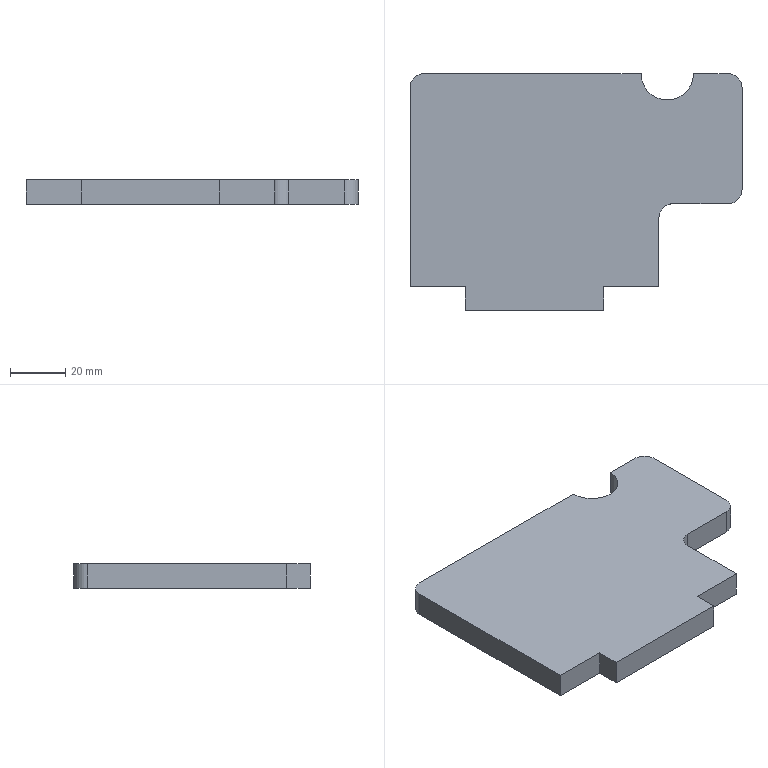Part | SolidWorks | features FlatPattern 1, SMBaseFlange 1, SheetMetal 1 | 1 solid | 18 faces | box 120 x 85.5 x 9 mm | volume 77513 mm3 | plane 13 | cylinder 5 | commonest cylinder face diameters 10 x4 19 x1
STEP:
#1=CARTESIAN_POINT('',(-433.387,-38.303,0.));
#2=VERTEX_POINT('',#1);
#3=CARTESIAN_POINT('',(-438.387,-33.303,0.));
#4=VERTEX_POINT('',#3);
#5=CARTESIAN_POINT('',(-438.387,-38.303,0.));
#6=DIRECTION('',(0.,0.,1.));
#7=DIRECTION('',(-1.,0.,0.));
#8=AXIS2_PLACEMENT_3D('',#5,#6,#7);
#9=CIRCLE('',#8,5.);
#10=EDGE_CURVE('',#2,#4,#9,.T.);
#11=ORIENTED_EDGE('',*,*,#10,.F.);
#12=CARTESIAN_POINT('',(-433.387,-38.303,-9.));
#13=VERTEX_POINT('',#12);
#14=CARTESIAN_POINT('',(-433.387,-38.303,-9.));
#15=DIRECTION('',(0.,0.,1.));
#16=VECTOR('',#15,1000.);
#17=LINE('',#14,#16);
#18=EDGE_CURVE('',#13,#2,#17,.T.);
#19=ORIENTED_EDGE('',*,*,#18,.F.);
#20=CARTESIAN_POINT('',(-438.387,-33.303,-9.));
#21=VERTEX_POINT('',#20);
#22=CARTESIAN_POINT('',(-438.387,-38.303,-9.));
#23=DIRECTION('',(0.,0.,1.));
#24=DIRECTION('',(-1.,0.,0.));
#25=AXIS2_PLACEMENT_3D('',#22,#23,#24);
#26=CIRCLE('',#25,5.);
#27=EDGE_CURVE('',#13,#21,#26,.T.);
#28=ORIENTED_EDGE('',*,*,#27,.T.);
#29=CARTESIAN_POINT('',(-438.387,-33.303,-9.));
#30=DIRECTION('',(0.,0.,1.));
#31=VECTOR('',#30,1000.);
#32=LINE('',#29,#31);
#33=EDGE_CURVE('',#21,#4,#32,.T.);
#34=ORIENTED_EDGE('',*,*,#33,.T.);
#35=EDGE_LOOP('',(#11,#19,#28,#34));
#36=FACE_OUTER_BOUND('',#35,.T.);
#37=CARTESIAN_POINT('',(-438.387,-38.303,-9.));
#38=DIRECTION('',(0.,0.,1.));
#39=DIRECTION('',(1.,0.,0.));
#40=AXIS2_PLACEMENT_3D('',#37,#38,#39);
#41=CYLINDRICAL_SURFACE('',#40,5.);
#42=ADVANCED_FACE('',(#36),#41,.T.);
#43=CARTESIAN_POINT('',(-433.387,-75.303,0.));
#44=VERTEX_POINT('',#43);
#45=CARTESIAN_POINT('',(-433.387,-75.303,0.));
#46=DIRECTION('',(0.,1.,0.));
#47=VECTOR('',#46,1000.);
#48=LINE('',#45,#47);
#49=EDGE_CURVE('',#44,#2,#48,.T.);
#50=ORIENTED_EDGE('',*,*,#49,.F.);
#51=CARTESIAN_POINT('',(-433.387,-75.303,-9.));
#52=VERTEX_POINT('',#51);
#53=CARTESIAN_POINT('',(-433.387,-75.303,-9.));
#54=DIRECTION('',(0.,0.,1.));
#55=VECTOR('',#54,1000.);
#56=LINE('',#53,#55);
#57=EDGE_CURVE('',#52,#44,#56,.T.);
#58=ORIENTED_EDGE('',*,*,#57,.F.);
#59=CARTESIAN_POINT('',(-433.387,-75.303,-9.));
#60=DIRECTION('',(0.,1.,0.));
#61=VECTOR('',#60,1000.);
#62=LINE('',#59,#61);
#63=EDGE_CURVE('',#52,#13,#62,.T.);
#64=ORIENTED_EDGE('',*,*,#63,.T.);
#65=ORIENTED_EDGE('',*,*,#18,.T.);
#66=EDGE_LOOP('',(#50,#58,#64,#65));
#67=FACE_OUTER_BOUND('',#66,.T.);
#68=CARTESIAN_POINT('',(-433.387,-75.303,-9.));
#69=DIRECTION('',(1.,0.,0.));
#70=DIRECTION('',(0.,0.,-1.));
#71=AXIS2_PLACEMENT_3D('',#68,#69,#70);
#72=PLANE('',#71);
#73=ADVANCED_FACE('',(#67),#72,.T.);
#74=CARTESIAN_POINT('',(-438.387,-80.303,0.));
#75=VERTEX_POINT('',#74);
#76=CARTESIAN_POINT('',(-438.387,-75.303,0.));
#77=DIRECTION('',(0.,0.,1.));
#78=DIRECTION('',(1.,0.,0.));
#79=AXIS2_PLACEMENT_3D('',#76,#77,#78);
#80=CIRCLE('',#79,5.);
#81=EDGE_CURVE('',#75,#44,#80,.T.);
#82=ORIENTED_EDGE('',*,*,#81,.F.);
#83=CARTESIAN_POINT('',(-438.387,-80.303,-9.));
#84=VERTEX_POINT('',#83);
#85=CARTESIAN_POINT('',(-438.387,-80.303,-9.));
#86=DIRECTION('',(0.,0.,1.));
#87=VECTOR('',#86,1000.);
#88=LINE('',#85,#87);
#89=EDGE_CURVE('',#84,#75,#88,.T.);
#90=ORIENTED_EDGE('',*,*,#89,.F.);
#91=CARTESIAN_POINT('',(-438.387,-75.303,-9.));
#92=DIRECTION('',(0.,0.,1.));
#93=DIRECTION('',(1.,0.,0.));
#94=AXIS2_PLACEMENT_3D('',#91,#92,#93);
#95=CIRCLE('',#94,5.);
#96=EDGE_CURVE('',#84,#52,#95,.T.);
#97=ORIENTED_EDGE('',*,*,#96,.T.);
#98=ORIENTED_EDGE('',*,*,#57,.T.);
#99=EDGE_LOOP('',(#82,#90,#97,#98));
#100=FACE_OUTER_BOUND('',#99,.T.);
#101=CARTESIAN_POINT('',(-438.387,-75.303,-9.));
#102=DIRECTION('',(0.,0.,1.));
#103=DIRECTION('',(1.,0.,0.));
#104=AXIS2_PLACEMENT_3D('',#101,#102,#103);
#105=CYLINDRICAL_SURFACE('',#104,5.);
#106=ADVANCED_FACE('',(#100),#105,.T.);
#107=CARTESIAN_POINT('',(-458.387,-80.303,0.));
#108=VERTEX_POINT('',#107);
#109=CARTESIAN_POINT('',(-458.387,-80.303,0.));
#110=DIRECTION('',(1.,0.,0.));
#111=VECTOR('',#110,1000.);
#112=LINE('',#109,#111);
#113=EDGE_CURVE('',#108,#75,#112,.T.);
#114=ORIENTED_EDGE('',*,*,#113,.F.);
#115=CARTESIAN_POINT('',(-458.387,-80.303,-9.));
#116=VERTEX_POINT('',#115);
#117=CARTESIAN_POINT('',(-458.387,-80.303,-9.));
#118=DIRECTION('',(0.,0.,1.));
#119=VECTOR('',#118,1000.);
#120=LINE('',#117,#119);
#121=EDGE_CURVE('',#116,#108,#120,.T.);
#122=ORIENTED_EDGE('',*,*,#121,.F.);
#123=CARTESIAN_POINT('',(-458.387,-80.303,-9.));
#124=DIRECTION('',(1.,0.,0.));
#125=VECTOR('',#124,1000.);
#126=LINE('',#123,#125);
#127=EDGE_CURVE('',#116,#84,#126,.T.);
#128=ORIENTED_EDGE('',*,*,#127,.T.);
#129=ORIENTED_EDGE('',*,*,#89,.T.);
#130=EDGE_LOOP('',(#114,#122,#128,#129));
#131=FACE_OUTER_BOUND('',#130,.T.);
#132=CARTESIAN_POINT('',(-458.387,-80.303,-9.));
#133=DIRECTION('',(0.,-1.,0.));
#134=DIRECTION('',(0.,0.,-1.));
#135=AXIS2_PLACEMENT_3D('',#132,#133,#134);
#136=PLANE('',#135);
#137=ADVANCED_FACE('',(#131),#136,.T.);
#138=CARTESIAN_POINT('',(-463.387,-85.303,0.));
#139=VERTEX_POINT('',#138);
#140=CARTESIAN_POINT('',(-458.387,-85.303,0.));
#141=DIRECTION('',(0.,0.,-1.));
#142=DIRECTION('',(-1.,0.,0.));
#143=AXIS2_PLACEMENT_3D('',#140,#141,#142);
#144=CIRCLE('',#143,5.);
#145=EDGE_CURVE('',#139,#108,#144,.T.);
#146=ORIENTED_EDGE('',*,*,#145,.F.);
#147=CARTESIAN_POINT('',(-463.387,-85.303,-9.));
#148=VERTEX_POINT('',#147);
#149=CARTESIAN_POINT('',(-463.387,-85.303,-9.));
#150=DIRECTION('',(0.,0.,1.));
#151=VECTOR('',#150,1000.);
#152=LINE('',#149,#151);
#153=EDGE_CURVE('',#148,#139,#152,.T.);
#154=ORIENTED_EDGE('',*,*,#153,.F.);
#155=CARTESIAN_POINT('',(-458.387,-85.303,-9.));
#156=DIRECTION('',(0.,0.,-1.));
#157=DIRECTION('',(-1.,0.,0.));
#158=AXIS2_PLACEMENT_3D('',#155,#156,#157);
#159=CIRCLE('',#158,5.);
#160=EDGE_CURVE('',#148,#116,#159,.T.);
#161=ORIENTED_EDGE('',*,*,#160,.T.);
#162=ORIENTED_EDGE('',*,*,#121,.T.);
#163=EDGE_LOOP('',(#146,#154,#161,#162));
#164=FACE_OUTER_BOUND('',#163,.T.);
#165=CARTESIAN_POINT('',(-458.387,-85.303,-9.));
#166=DIRECTION('',(0.,0.,1.));
#167=DIRECTION('',(1.,0.,0.));
#168=AXIS2_PLACEMENT_3D('',#165,#166,#167);
#169=CYLINDRICAL_SURFACE('',#168,5.);
#170=ADVANCED_FACE('',(#164),#169,.F.);
#171=CARTESIAN_POINT('',(-463.387,-110.303,0.));
#172=VERTEX_POINT('',#171);
#173=CARTESIAN_POINT('',(-463.387,-110.303,0.));
#174=DIRECTION('',(0.,1.,0.));
#175=VECTOR('',#174,1000.);
#176=LINE('',#173,#175);
#177=EDGE_CURVE('',#172,#139,#176,.T.);
#178=ORIENTED_EDGE('',*,*,#177,.F.);
#179=CARTESIAN_POINT('',(-463.387,-110.303,-9.));
#180=VERTEX_POINT('',#179);
#181=CARTESIAN_POINT('',(-463.387,-110.303,-9.));
#182=DIRECTION('',(0.,0.,1.));
#183=VECTOR('',#182,1000.);
#184=LINE('',#181,#183);
#185=EDGE_CURVE('',#180,#172,#184,.T.);
#186=ORIENTED_EDGE('',*,*,#185,.F.);
#187=CARTESIAN_POINT('',(-463.387,-110.303,-9.));
#188=DIRECTION('',(0.,1.,0.));
#189=VECTOR('',#188,1000.);
#190=LINE('',#187,#189);
#191=EDGE_CURVE('',#180,#148,#190,.T.);
#192=ORIENTED_EDGE('',*,*,#191,.T.);
#193=ORIENTED_EDGE('',*,*,#153,.T.);
#194=EDGE_LOOP('',(#178,#186,#192,#193));
#195=FACE_OUTER_BOUND('',#194,.T.);
#196=CARTESIAN_POINT('',(-463.387,-110.303,-9.));
#197=DIRECTION('',(1.,0.,0.));
#198=DIRECTION('',(0.,0.,-1.));
#199=AXIS2_PLACEMENT_3D('',#196,#197,#198);
#200=PLANE('',#199);
#201=ADVANCED_FACE('',(#195),#200,.T.);
#202=CARTESIAN_POINT('',(-483.387,-110.303,0.));
#203=VERTEX_POINT('',#202);
#204=CARTESIAN_POINT('',(-483.387,-110.303,0.));
#205=DIRECTION('',(1.,0.,0.));
#206=VECTOR('',#205,1000.);
#207=LINE('',#204,#206);
#208=EDGE_CURVE('',#203,#172,#207,.T.);
#209=ORIENTED_EDGE('',*,*,#208,.F.);
#210=CARTESIAN_POINT('',(-483.387,-110.303,-9.));
#211=VERTEX_POINT('',#210);
#212=CARTESIAN_POINT('',(-483.387,-110.303,-9.));
#213=DIRECTION('',(0.,0.,1.));
#214=VECTOR('',#213,1000.);
#215=LINE('',#212,#214);
#216=EDGE_CURVE('',#211,#203,#215,.T.);
#217=ORIENTED_EDGE('',*,*,#216,.F.);
#218=CARTESIAN_POINT('',(-483.387,-110.303,-9.));
#219=DIRECTION('',(1.,0.,0.));
#220=VECTOR('',#219,1000.);
#221=LINE('',#218,#220);
#222=EDGE_CURVE('',#211,#180,#221,.T.);
#223=ORIENTED_EDGE('',*,*,#222,.T.);
#224=ORIENTED_EDGE('',*,*,#185,.T.);
#225=EDGE_LOOP('',(#209,#217,#223,#224));
#226=FACE_OUTER_BOUND('',#225,.T.);
#227=CARTESIAN_POINT('',(-483.387,-110.303,-9.));
#228=DIRECTION('',(0.,-1.,0.));
#229=DIRECTION('',(0.,0.,-1.));
#230=AXIS2_PLACEMENT_3D('',#227,#228,#229);
#231=PLANE('',#230);
#232=ADVANCED_FACE('',(#226),#231,.T.);
#233=CARTESIAN_POINT('',(-483.387,-118.803,0.));
#234=VERTEX_POINT('',#233);
#235=CARTESIAN_POINT('',(-483.387,-118.803,0.));
#236=DIRECTION('',(0.,1.,0.));
#237=VECTOR('',#236,1000.);
#238=LINE('',#235,#237);
#239=EDGE_CURVE('',#234,#203,#238,.T.);
#240=ORIENTED_EDGE('',*,*,#239,.F.);
#241=CARTESIAN_POINT('',(-483.387,-118.803,-9.));
#242=VERTEX_POINT('',#241);
#243=CARTESIAN_POINT('',(-483.387,-118.803,-9.));
#244=DIRECTION('',(0.,0.,1.));
#245=VECTOR('',#244,1000.);
#246=LINE('',#243,#245);
#247=EDGE_CURVE('',#242,#234,#246,.T.);
#248=ORIENTED_EDGE('',*,*,#247,.F.);
#249=CARTESIAN_POINT('',(-483.387,-118.803,-9.));
#250=DIRECTION('',(0.,1.,0.));
#251=VECTOR('',#250,1000.);
#252=LINE('',#249,#251);
#253=EDGE_CURVE('',#242,#211,#252,.T.);
#254=ORIENTED_EDGE('',*,*,#253,.T.);
#255=ORIENTED_EDGE('',*,*,#216,.T.);
#256=EDGE_LOOP('',(#240,#248,#254,#255));
#257=FACE_OUTER_BOUND('',#256,.T.);
#258=CARTESIAN_POINT('',(-483.387,-118.803,-9.));
#259=DIRECTION('',(1.,0.,0.));
#260=DIRECTION('',(0.,0.,-1.));
#261=AXIS2_PLACEMENT_3D('',#258,#259,#260);
#262=PLANE('',#261);
#263=ADVANCED_FACE('',(#257),#262,.T.);
#264=CARTESIAN_POINT('',(-533.387,-118.803,0.));
#265=VERTEX_POINT('',#264);
#266=CARTESIAN_POINT('',(-533.387,-118.803,0.));
#267=DIRECTION('',(1.,0.,0.));
#268=VECTOR('',#267,1000.);
#269=LINE('',#266,#268);
#270=EDGE_CURVE('',#265,#234,#269,.T.);
#271=ORIENTED_EDGE('',*,*,#270,.F.);
#272=CARTESIAN_POINT('',(-533.387,-118.803,-9.));
#273=VERTEX_POINT('',#272);
#274=CARTESIAN_POINT('',(-533.387,-118.803,-9.));
#275=DIRECTION('',(0.,0.,1.));
#276=VECTOR('',#275,1000.);
#277=LINE('',#274,#276);
#278=EDGE_CURVE('',#273,#265,#277,.T.);
#279=ORIENTED_EDGE('',*,*,#278,.F.);
#280=CARTESIAN_POINT('',(-533.387,-118.803,-9.));
#281=DIRECTION('',(1.,0.,0.));
#282=VECTOR('',#281,1000.);
#283=LINE('',#280,#282);
#284=EDGE_CURVE('',#273,#242,#283,.T.);
#285=ORIENTED_EDGE('',*,*,#284,.T.);
#286=ORIENTED_EDGE('',*,*,#247,.T.);
#287=EDGE_LOOP('',(#271,#279,#285,#286));
#288=FACE_OUTER_BOUND('',#287,.T.);
#289=CARTESIAN_POINT('',(-533.387,-118.803,-9.));
#290=DIRECTION('',(0.,-1.,0.));
#291=DIRECTION('',(0.,0.,-1.));
#292=AXIS2_PLACEMENT_3D('',#289,#290,#291);
#293=PLANE('',#292);
#294=ADVANCED_FACE('',(#288),#293,.T.);
#295=CARTESIAN_POINT('',(-533.387,-110.303,0.));
#296=VERTEX_POINT('',#295);
#297=CARTESIAN_POINT('',(-533.387,-110.303,0.));
#298=DIRECTION('',(0.,-1.,0.));
#299=VECTOR('',#298,1000.);
#300=LINE('',#297,#299);
#301=EDGE_CURVE('',#296,#265,#300,.T.);
#302=ORIENTED_EDGE('',*,*,#301,.F.);
#303=CARTESIAN_POINT('',(-533.387,-110.303,-9.));
#304=VERTEX_POINT('',#303);
#305=CARTESIAN_POINT('',(-533.387,-110.303,-9.));
#306=DIRECTION('',(0.,0.,1.));
#307=VECTOR('',#306,1000.);
#308=LINE('',#305,#307);
#309=EDGE_CURVE('',#304,#296,#308,.T.);
#310=ORIENTED_EDGE('',*,*,#309,.F.);
#311=CARTESIAN_POINT('',(-533.387,-110.303,-9.));
#312=DIRECTION('',(0.,-1.,0.));
#313=VECTOR('',#312,1000.);
#314=LINE('',#311,#313);
#315=EDGE_CURVE('',#304,#273,#314,.T.);
#316=ORIENTED_EDGE('',*,*,#315,.T.);
#317=ORIENTED_EDGE('',*,*,#278,.T.);
#318=EDGE_LOOP('',(#302,#310,#316,#317));
#319=FACE_OUTER_BOUND('',#318,.T.);
#320=CARTESIAN_POINT('',(-533.387,-110.303,-9.));
#321=DIRECTION('',(-1.,0.,0.));
#322=DIRECTION('',(0.,0.,1.));
#323=AXIS2_PLACEMENT_3D('',#320,#321,#322);
#324=PLANE('',#323);
#325=ADVANCED_FACE('',(#319),#324,.T.);
#326=CARTESIAN_POINT('',(-553.387,-110.303,0.));
#327=VERTEX_POINT('',#326);
#328=CARTESIAN_POINT('',(-553.387,-110.303,0.));
#329=DIRECTION('',(1.,0.,0.));
#330=VECTOR('',#329,1000.);
#331=LINE('',#328,#330);
#332=EDGE_CURVE('',#327,#296,#331,.T.);
#333=ORIENTED_EDGE('',*,*,#332,.F.);
#334=CARTESIAN_POINT('',(-553.387,-110.303,-9.));
#335=VERTEX_POINT('',#334);
#336=CARTESIAN_POINT('',(-553.387,-110.303,-9.));
#337=DIRECTION('',(0.,0.,1.));
#338=VECTOR('',#337,1000.);
#339=LINE('',#336,#338);
#340=EDGE_CURVE('',#335,#327,#339,.T.);
#341=ORIENTED_EDGE('',*,*,#340,.F.);
#342=CARTESIAN_POINT('',(-553.387,-110.303,-9.));
#343=DIRECTION('',(1.,0.,0.));
#344=VECTOR('',#343,1000.);
#345=LINE('',#342,#344);
#346=EDGE_CURVE('',#335,#304,#345,.T.);
#347=ORIENTED_EDGE('',*,*,#346,.T.);
#348=ORIENTED_EDGE('',*,*,#309,.T.);
#349=EDGE_LOOP('',(#333,#341,#347,#348));
#350=FACE_OUTER_BOUND('',#349,.T.);
#351=CARTESIAN_POINT('',(-553.387,-110.303,-9.));
#352=DIRECTION('',(0.,-1.,0.));
#353=DIRECTION('',(0.,0.,-1.));
#354=AXIS2_PLACEMENT_3D('',#351,#352,#353);
#355=PLANE('',#354);
#356=ADVANCED_FACE('',(#350),#355,.T.);
#357=CARTESIAN_POINT('',(-553.387,-38.303,0.));
#358=VERTEX_POINT('',#357);
#359=CARTESIAN_POINT('',(-553.387,-38.303,0.));
#360=DIRECTION('',(0.,-1.,0.));
#361=VECTOR('',#360,1000.);
#362=LINE('',#359,#361);
#363=EDGE_CURVE('',#358,#327,#362,.T.);
#364=ORIENTED_EDGE('',*,*,#363,.F.);
#365=CARTESIAN_POINT('',(-553.387,-38.303,-9.));
#366=VERTEX_POINT('',#365);
#367=CARTESIAN_POINT('',(-553.387,-38.303,-9.));
#368=DIRECTION('',(0.,0.,1.));
#369=VECTOR('',#368,1000.);
#370=LINE('',#367,#369);
#371=EDGE_CURVE('',#366,#358,#370,.T.);
#372=ORIENTED_EDGE('',*,*,#371,.F.);
#373=CARTESIAN_POINT('',(-553.387,-38.303,-9.));
#374=DIRECTION('',(0.,-1.,0.));
#375=VECTOR('',#374,1000.);
#376=LINE('',#373,#375);
#377=EDGE_CURVE('',#366,#335,#376,.T.);
#378=ORIENTED_EDGE('',*,*,#377,.T.);
#379=ORIENTED_EDGE('',*,*,#340,.T.);
#380=EDGE_LOOP('',(#364,#372,#378,#379));
#381=FACE_OUTER_BOUND('',#380,.T.);
#382=CARTESIAN_POINT('',(-553.387,-38.303,-9.));
#383=DIRECTION('',(-1.,0.,0.));
#384=DIRECTION('',(0.,0.,1.));
#385=AXIS2_PLACEMENT_3D('',#382,#383,#384);
#386=PLANE('',#385);
#387=ADVANCED_FACE('',(#381),#386,.T.);
#388=CARTESIAN_POINT('',(-548.387,-33.303,0.));
#389=VERTEX_POINT('',#388);
#390=CARTESIAN_POINT('',(-548.387,-38.303,0.));
#391=DIRECTION('',(0.,0.,1.));
#392=DIRECTION('',(1.,0.,0.));
#393=AXIS2_PLACEMENT_3D('',#390,#391,#392);
#394=CIRCLE('',#393,5.);
#395=EDGE_CURVE('',#389,#358,#394,.T.);
#396=ORIENTED_EDGE('',*,*,#395,.F.);
#397=CARTESIAN_POINT('',(-548.387,-33.303,-9.));
#398=VERTEX_POINT('',#397);
#399=CARTESIAN_POINT('',(-548.387,-33.303,-9.));
#400=DIRECTION('',(0.,0.,1.));
#401=VECTOR('',#400,1000.);
#402=LINE('',#399,#401);
#403=EDGE_CURVE('',#398,#389,#402,.T.);
#404=ORIENTED_EDGE('',*,*,#403,.F.);
#405=CARTESIAN_POINT('',(-548.387,-38.303,-9.));
#406=DIRECTION('',(0.,0.,1.));
#407=DIRECTION('',(1.,0.,0.));
#408=AXIS2_PLACEMENT_3D('',#405,#406,#407);
#409=CIRCLE('',#408,5.);
#410=EDGE_CURVE('',#398,#366,#409,.T.);
#411=ORIENTED_EDGE('',*,*,#410,.T.);
#412=ORIENTED_EDGE('',*,*,#371,.T.);
#413=EDGE_LOOP('',(#396,#404,#411,#412));
#414=FACE_OUTER_BOUND('',#413,.T.);
#415=CARTESIAN_POINT('',(-548.387,-38.303,-9.));
#416=DIRECTION('',(0.,0.,1.));
#417=DIRECTION('',(1.,0.,0.));
#418=AXIS2_PLACEMENT_3D('',#415,#416,#417);
#419=CYLINDRICAL_SURFACE('',#418,5.);
#420=ADVANCED_FACE('',(#414),#419,.T.);
#421=CARTESIAN_POINT('',(-469.887,-33.303,0.));
#422=VERTEX_POINT('',#421);
#423=CARTESIAN_POINT('',(-469.887,-33.303,0.));
#424=DIRECTION('',(-1.,0.,0.));
#425=VECTOR('',#424,1000.);
#426=LINE('',#423,#425);
#427=EDGE_CURVE('',#422,#389,#426,.T.);
#428=ORIENTED_EDGE('',*,*,#427,.F.);
#429=CARTESIAN_POINT('',(-469.887,-33.303,-9.));
#430=VERTEX_POINT('',#429);
#431=CARTESIAN_POINT('',(-469.887,-33.303,-9.));
#432=DIRECTION('',(0.,0.,1.));
#433=VECTOR('',#432,1000.);
#434=LINE('',#431,#433);
#435=EDGE_CURVE('',#430,#422,#434,.T.);
#436=ORIENTED_EDGE('',*,*,#435,.F.);
#437=CARTESIAN_POINT('',(-469.887,-33.303,-9.));
#438=DIRECTION('',(-1.,0.,0.));
#439=VECTOR('',#438,1000.);
#440=LINE('',#437,#439);
#441=EDGE_CURVE('',#430,#398,#440,.T.);
#442=ORIENTED_EDGE('',*,*,#441,.T.);
#443=ORIENTED_EDGE('',*,*,#403,.T.);
#444=EDGE_LOOP('',(#428,#436,#442,#443));
#445=FACE_OUTER_BOUND('',#444,.T.);
#446=CARTESIAN_POINT('',(-469.887,-33.303,-9.));
#447=DIRECTION('',(0.,1.,0.));
#448=DIRECTION('',(-1.,0.,0.));
#449=AXIS2_PLACEMENT_3D('',#446,#447,#448);
#450=PLANE('',#449);
#451=ADVANCED_FACE('',(#445),#450,.T.);
#452=CARTESIAN_POINT('',(-450.887,-33.303,0.));
#453=VERTEX_POINT('',#452);
#454=CARTESIAN_POINT('',(-460.387,-33.303,0.));
#455=DIRECTION('',(0.,0.,-1.));
#456=DIRECTION('',(1.,0.,0.));
#457=AXIS2_PLACEMENT_3D('',#454,#455,#456);
#458=CIRCLE('',#457,9.5);
#459=EDGE_CURVE('',#453,#422,#458,.T.);
#460=ORIENTED_EDGE('',*,*,#459,.F.);
#461=CARTESIAN_POINT('',(-450.887,-33.303,-9.));
#462=VERTEX_POINT('',#461);
#463=CARTESIAN_POINT('',(-450.887,-33.303,-9.));
#464=DIRECTION('',(0.,0.,1.));
#465=VECTOR('',#464,1000.);
#466=LINE('',#463,#465);
#467=EDGE_CURVE('',#462,#453,#466,.T.);
#468=ORIENTED_EDGE('',*,*,#467,.F.);
#469=CARTESIAN_POINT('',(-460.387,-33.303,-9.));
#470=DIRECTION('',(0.,0.,-1.));
#471=DIRECTION('',(1.,0.,0.));
#472=AXIS2_PLACEMENT_3D('',#469,#470,#471);
#473=CIRCLE('',#472,9.5);
#474=EDGE_CURVE('',#462,#430,#473,.T.);
#475=ORIENTED_EDGE('',*,*,#474,.T.);
#476=ORIENTED_EDGE('',*,*,#435,.T.);
#477=EDGE_LOOP('',(#460,#468,#475,#476));
#478=FACE_OUTER_BOUND('',#477,.T.);
#479=CARTESIAN_POINT('',(-460.387,-33.303,-9.));
#480=DIRECTION('',(0.,0.,1.));
#481=DIRECTION('',(1.,0.,0.));
#482=AXIS2_PLACEMENT_3D('',#479,#480,#481);
#483=CYLINDRICAL_SURFACE('',#482,9.5);
#484=ADVANCED_FACE('',(#478),#483,.F.);
#485=CARTESIAN_POINT('',(-450.887,-33.303,0.));
#486=DIRECTION('',(-1.,0.,0.));
#487=VECTOR('',#486,1000.);
#488=LINE('',#485,#487);
#489=EDGE_CURVE('',#4,#453,#488,.T.);
#490=ORIENTED_EDGE('',*,*,#489,.F.);
#491=ORIENTED_EDGE('',*,*,#33,.F.);
#492=CARTESIAN_POINT('',(-450.887,-33.303,-9.));
#493=DIRECTION('',(-1.,0.,0.));
#494=VECTOR('',#493,1000.);
#495=LINE('',#492,#494);
#496=EDGE_CURVE('',#21,#462,#495,.T.);
#497=ORIENTED_EDGE('',*,*,#496,.T.);
#498=ORIENTED_EDGE('',*,*,#467,.T.);
#499=EDGE_LOOP('',(#490,#491,#497,#498));
#500=FACE_OUTER_BOUND('',#499,.T.);
#501=CARTESIAN_POINT('',(-450.887,-33.303,-9.));
#502=DIRECTION('',(0.,1.,0.));
#503=DIRECTION('',(-1.,0.,0.));
#504=AXIS2_PLACEMENT_3D('',#501,#502,#503);
#505=PLANE('',#504);
#506=ADVANCED_FACE('',(#500),#505,.T.);
#507=ORIENTED_EDGE('',*,*,#27,.F.);
#508=ORIENTED_EDGE('',*,*,#63,.F.);
#509=ORIENTED_EDGE('',*,*,#96,.F.);
#510=ORIENTED_EDGE('',*,*,#127,.F.);
#511=ORIENTED_EDGE('',*,*,#160,.F.);
#512=ORIENTED_EDGE('',*,*,#191,.F.);
#513=ORIENTED_EDGE('',*,*,#222,.F.);
#514=ORIENTED_EDGE('',*,*,#253,.F.);
#515=ORIENTED_EDGE('',*,*,#284,.F.);
#516=ORIENTED_EDGE('',*,*,#315,.F.);
#517=ORIENTED_EDGE('',*,*,#346,.F.);
#518=ORIENTED_EDGE('',*,*,#377,.F.);
#519=ORIENTED_EDGE('',*,*,#410,.F.);
#520=ORIENTED_EDGE('',*,*,#441,.F.);
#521=ORIENTED_EDGE('',*,*,#474,.F.);
#522=ORIENTED_EDGE('',*,*,#496,.F.);
#523=EDGE_LOOP('',(#507,#508,#509,#510,#511,#512,#513,#514,#515,#516,#517,#518,#519,#520,#521,#522));
#524=FACE_OUTER_BOUND('',#523,.T.);
#525=CARTESIAN_POINT('',(-438.387,-38.303,-9.));
#526=DIRECTION('',(0.,0.,-1.));
#527=DIRECTION('',(-1.,0.,0.));
#528=AXIS2_PLACEMENT_3D('',#525,#526,#527);
#529=PLANE('',#528);
#530=ADVANCED_FACE('',(#524),#529,.T.);
#531=ORIENTED_EDGE('',*,*,#10,.T.);
#532=ORIENTED_EDGE('',*,*,#489,.T.);
#533=ORIENTED_EDGE('',*,*,#459,.T.);
#534=ORIENTED_EDGE('',*,*,#427,.T.);
#535=ORIENTED_EDGE('',*,*,#395,.T.);
#536=ORIENTED_EDGE('',*,*,#363,.T.);
#537=ORIENTED_EDGE('',*,*,#332,.T.);
#538=ORIENTED_EDGE('',*,*,#301,.T.);
#539=ORIENTED_EDGE('',*,*,#270,.T.);
#540=ORIENTED_EDGE('',*,*,#239,.T.);
#541=ORIENTED_EDGE('',*,*,#208,.T.);
#542=ORIENTED_EDGE('',*,*,#177,.T.);
#543=ORIENTED_EDGE('',*,*,#145,.T.);
#544=ORIENTED_EDGE('',*,*,#113,.T.);
#545=ORIENTED_EDGE('',*,*,#81,.T.);
#546=ORIENTED_EDGE('',*,*,#49,.T.);
#547=EDGE_LOOP('',(#531,#532,#533,#534,#535,#536,#537,#538,#539,#540,#541,#542,#543,#544,#545,#546));
#548=FACE_OUTER_BOUND('',#547,.T.);
#549=CARTESIAN_POINT('',(-438.387,-38.303,0.));
#550=DIRECTION('',(0.,0.,-1.));
#551=DIRECTION('',(-1.,0.,0.));
#552=AXIS2_PLACEMENT_3D('',#549,#550,#551);
#553=PLANE('',#552);
#554=ADVANCED_FACE('',(#548),#553,.F.);
#555=CLOSED_SHELL('',(#42,#73,#106,#137,#170,#201,#232,#263,#294,#325,#356,#387,#420,#451,#484,#506,#530,#554));
#556=MANIFOLD_SOLID_BREP('',#555);
#557=CARTESIAN_POINT('',(0.,0.,0.));
#558=DIRECTION('',(0.,0.,1.));
#559=DIRECTION('',(1.,0.,0.));
#560=AXIS2_PLACEMENT_3D('',#557,#558,#559);
#561=(LENGTH_UNIT()NAMED_UNIT(*)SI_UNIT(.MILLI.,.METRE.));
#562=UNCERTAINTY_MEASURE_WITH_UNIT(LENGTH_MEASURE(0.00001),#561,'','');
#563=(NAMED_UNIT(*)PLANE_ANGLE_UNIT()SI_UNIT($,.RADIAN.));
#564=(NAMED_UNIT(*)SI_UNIT($,.STERADIAN.)SOLID_ANGLE_UNIT());
#565=(GEOMETRIC_REPRESENTATION_CONTEXT(3)GLOBAL_UNCERTAINTY_ASSIGNED_CONTEXT((#562))GLOBAL_UNIT_ASSIGNED_CONTEXT((#561,#563,#564))REPRESENTATION_CONTEXT('',''));
#566=ADVANCED_BREP_SHAPE_REPRESENTATION('',(#556,#560),#565);